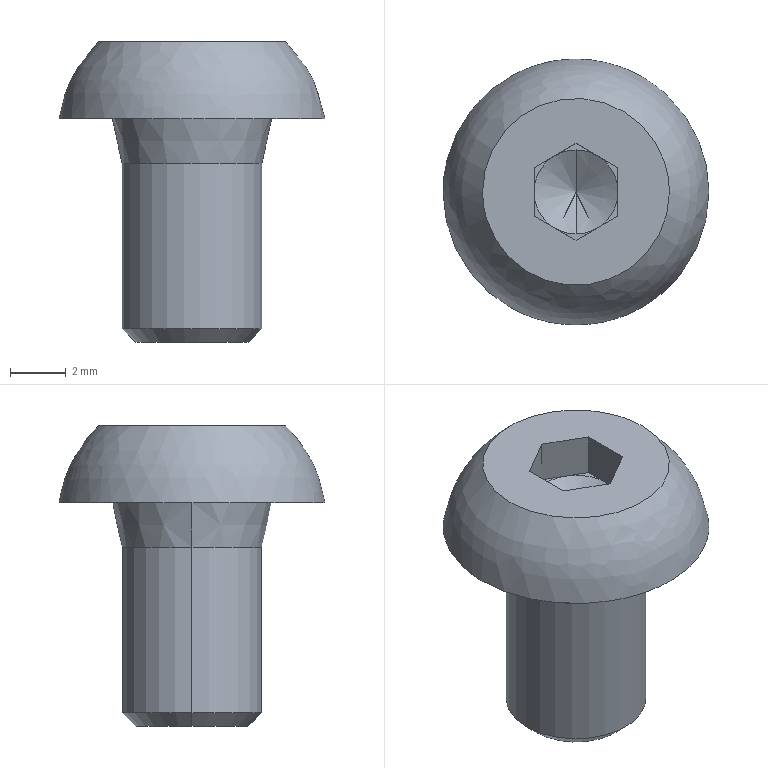Part | SolidWorks | features BaseBody 1 | 1 solid | 24 faces | box 9.5 x 9.5 x 10.75 mm | volume 302.249 mm3 | plane 15 | cone 6 | cylinder 2 | spline 1 | commonest cylinder face diameters 5 x2
STEP:
#1=CARTESIAN_POINT('',(2.5,0.,-5.91));
#2=VERTEX_POINT('',#1);
#3=CARTESIAN_POINT('',(-2.5,0.,-5.91));
#4=VERTEX_POINT('',#3);
#5=CARTESIAN_POINT('',(0.,0.,-5.91));
#6=DIRECTION('',(0.,0.,1.));
#7=DIRECTION('',(1.,0.,0.));
#8=AXIS2_PLACEMENT_3D('',#5,#6,#7);
#9=CIRCLE('',#8,2.5);
#10=EDGE_CURVE('',#2,#4,#9,.T.);
#11=ORIENTED_EDGE('',*,*,#10,.T.);
#12=CARTESIAN_POINT('',(-2.5,0.,0.));
#13=VERTEX_POINT('',#12);
#14=CARTESIAN_POINT('',(-2.5,0.,-6.4));
#15=DIRECTION('',(0.,0.,1.));
#16=VECTOR('',#15,1000.);
#17=LINE('',#14,#16);
#18=EDGE_CURVE('',#4,#13,#17,.T.);
#19=ORIENTED_EDGE('',*,*,#18,.T.);
#20=CARTESIAN_POINT('',(2.5,0.,0.));
#21=VERTEX_POINT('',#20);
#22=CARTESIAN_POINT('',(0.,0.,0.));
#23=DIRECTION('',(0.,0.,-1.));
#24=DIRECTION('',(1.,0.,0.));
#25=AXIS2_PLACEMENT_3D('',#22,#23,#24);
#26=CIRCLE('',#25,2.5);
#27=EDGE_CURVE('',#13,#21,#26,.T.);
#28=ORIENTED_EDGE('',*,*,#27,.T.);
#29=CARTESIAN_POINT('',(2.5,0.,-6.4));
#30=DIRECTION('',(0.,0.,1.));
#31=VECTOR('',#30,1000.);
#32=LINE('',#29,#31);
#33=EDGE_CURVE('',#2,#21,#32,.T.);
#34=ORIENTED_EDGE('',*,*,#33,.F.);
#35=EDGE_LOOP('',(#11,#19,#28,#34));
#36=FACE_OUTER_BOUND('',#35,.T.);
#37=CARTESIAN_POINT('',(0.,0.,-6.4));
#38=DIRECTION('',(0.,0.,1.));
#39=DIRECTION('',(1.,0.,0.));
#40=AXIS2_PLACEMENT_3D('',#37,#38,#39);
#41=CYLINDRICAL_SURFACE('',#40,2.5);
#42=ADVANCED_FACE('',(#36),#41,.T.);
#43=ORIENTED_EDGE('',*,*,#27,.F.);
#44=CARTESIAN_POINT('',(-2.85,0.,1.6));
#45=VERTEX_POINT('',#44);
#46=CARTESIAN_POINT('',(-2.85,0.,1.6));
#47=DIRECTION('',(-0.2137,0.,0.9769));
#48=VECTOR('',#47,1000.);
#49=LINE('',#46,#48);
#50=EDGE_CURVE('',#13,#45,#49,.T.);
#51=ORIENTED_EDGE('',*,*,#50,.T.);
#52=CARTESIAN_POINT('',(2.85,0.,1.6));
#53=VERTEX_POINT('',#52);
#54=CARTESIAN_POINT('',(0.,0.,1.6));
#55=DIRECTION('',(0.,0.,-1.));
#56=DIRECTION('',(1.,0.,0.));
#57=AXIS2_PLACEMENT_3D('',#54,#55,#56);
#58=CIRCLE('',#57,2.85);
#59=EDGE_CURVE('',#45,#53,#58,.T.);
#60=ORIENTED_EDGE('',*,*,#59,.T.);
#61=CARTESIAN_POINT('',(2.85,0.,1.6));
#62=DIRECTION('',(0.2137,0.,0.9769));
#63=VECTOR('',#62,1000.);
#64=LINE('',#61,#63);
#65=EDGE_CURVE('',#21,#53,#64,.T.);
#66=ORIENTED_EDGE('',*,*,#65,.F.);
#67=EDGE_LOOP('',(#43,#51,#60,#66));
#68=FACE_OUTER_BOUND('',#67,.T.);
#69=CARTESIAN_POINT('',(0.,0.,1.6));
#70=DIRECTION('',(0.,0.,1.));
#71=DIRECTION('',(1.,0.,0.));
#72=AXIS2_PLACEMENT_3D('',#69,#70,#71);
#73=CONICAL_SURFACE('',#72,2.85,0.2154);
#74=ADVANCED_FACE('',(#68),#73,.T.);
#75=CARTESIAN_POINT('',(2.009,0.,-6.4));
#76=VERTEX_POINT('',#75);
#77=CARTESIAN_POINT('',(-2.009,0.,-6.4));
#78=VERTEX_POINT('',#77);
#79=CARTESIAN_POINT('',(0.,0.,-6.4));
#80=DIRECTION('',(0.,0.,1.));
#81=DIRECTION('',(1.,0.,0.));
#82=AXIS2_PLACEMENT_3D('',#79,#80,#81);
#83=CIRCLE('',#82,2.009);
#84=EDGE_CURVE('',#76,#78,#83,.T.);
#85=ORIENTED_EDGE('',*,*,#84,.T.);
#86=CARTESIAN_POINT('',(-2.5,0.,-5.91));
#87=DIRECTION('',(-0.7071,0.,0.7071));
#88=VECTOR('',#87,1000.);
#89=LINE('',#86,#88);
#90=EDGE_CURVE('',#78,#4,#89,.T.);
#91=ORIENTED_EDGE('',*,*,#90,.T.);
#92=ORIENTED_EDGE('',*,*,#10,.F.);
#93=CARTESIAN_POINT('',(2.5,0.,-5.91));
#94=DIRECTION('',(0.7071,0.,0.7071));
#95=VECTOR('',#94,1000.);
#96=LINE('',#93,#95);
#97=EDGE_CURVE('',#76,#2,#96,.T.);
#98=ORIENTED_EDGE('',*,*,#97,.F.);
#99=EDGE_LOOP('',(#85,#91,#92,#98));
#100=FACE_OUTER_BOUND('',#99,.T.);
#101=CARTESIAN_POINT('',(0.,0.,-5.91));
#102=DIRECTION('',(0.,0.,1.));
#103=DIRECTION('',(1.,0.,0.));
#104=AXIS2_PLACEMENT_3D('',#101,#102,#103);
#105=CONICAL_SURFACE('',#104,2.5,0.7854);
#106=ADVANCED_FACE('',(#100),#105,.T.);
#107=CARTESIAN_POINT('',(0.,0.,1.924));
#108=VERTEX_POINT('',#107);
#109=CARTESIAN_POINT('',(0.,-1.5,2.79));
#110=VERTEX_POINT('',#109);
#111=CARTESIAN_POINT('',(0.,-1.5,2.79));
#112=DIRECTION('',(0.,-0.866,0.5));
#113=VECTOR('',#112,1000.);
#114=LINE('',#111,#113);
#115=EDGE_CURVE('',#108,#110,#114,.T.);
#116=ORIENTED_EDGE('',*,*,#115,.F.);
#117=CARTESIAN_POINT('',(0.,1.5,2.79));
#118=VERTEX_POINT('',#117);
#119=CARTESIAN_POINT('',(0.,1.5,2.79));
#120=DIRECTION('',(0.,0.866,0.5));
#121=VECTOR('',#120,1000.);
#122=LINE('',#119,#121);
#123=EDGE_CURVE('',#108,#118,#122,.T.);
#124=ORIENTED_EDGE('',*,*,#123,.T.);
#125=CARTESIAN_POINT('',(-0.75,1.299,2.79));
#126=VERTEX_POINT('',#125);
#127=CARTESIAN_POINT('',(0.,0.,2.79));
#128=DIRECTION('',(0.,0.,-1.));
#129=DIRECTION('',(0.,-1.,0.));
#130=AXIS2_PLACEMENT_3D('',#127,#128,#129);
#131=CIRCLE('',#130,1.5);
#132=EDGE_CURVE('',#126,#118,#131,.T.);
#133=ORIENTED_EDGE('',*,*,#132,.F.);
#134=CARTESIAN_POINT('',(-1.5,0.,2.79));
#135=VERTEX_POINT('',#134);
#136=CARTESIAN_POINT('',(0.,0.,2.79));
#137=DIRECTION('',(0.,0.,-1.));
#138=DIRECTION('',(0.,-1.,0.));
#139=AXIS2_PLACEMENT_3D('',#136,#137,#138);
#140=CIRCLE('',#139,1.5);
#141=EDGE_CURVE('',#135,#126,#140,.T.);
#142=ORIENTED_EDGE('',*,*,#141,.F.);
#143=CARTESIAN_POINT('',(-0.75,-1.299,2.79));
#144=VERTEX_POINT('',#143);
#145=CARTESIAN_POINT('',(0.,0.,2.79));
#146=DIRECTION('',(0.,0.,-1.));
#147=DIRECTION('',(0.,-1.,0.));
#148=AXIS2_PLACEMENT_3D('',#145,#146,#147);
#149=CIRCLE('',#148,1.5);
#150=EDGE_CURVE('',#144,#135,#149,.T.);
#151=ORIENTED_EDGE('',*,*,#150,.F.);
#152=CARTESIAN_POINT('',(0.,0.,2.79));
#153=DIRECTION('',(0.,0.,-1.));
#154=DIRECTION('',(0.,-1.,0.));
#155=AXIS2_PLACEMENT_3D('',#152,#153,#154);
#156=CIRCLE('',#155,1.5);
#157=EDGE_CURVE('',#110,#144,#156,.T.);
#158=ORIENTED_EDGE('',*,*,#157,.F.);
#159=EDGE_LOOP('',(#116,#124,#133,#142,#151,#158));
#160=FACE_OUTER_BOUND('',#159,.T.);
#161=CARTESIAN_POINT('',(0.,0.,2.79));
#162=DIRECTION('',(0.,0.,1.));
#163=DIRECTION('',(0.,-1.,0.));
#164=AXIS2_PLACEMENT_3D('',#161,#162,#163);
#165=CONICAL_SURFACE('',#164,1.5,1.047);
#166=ADVANCED_FACE('',(#160),#165,.F.);
#167=ORIENTED_EDGE('',*,*,#18,.F.);
#168=CARTESIAN_POINT('',(0.,0.,-5.91));
#169=DIRECTION('',(0.,0.,1.));
#170=DIRECTION('',(1.,0.,0.));
#171=AXIS2_PLACEMENT_3D('',#168,#169,#170);
#172=CIRCLE('',#171,2.5);
#173=EDGE_CURVE('',#4,#2,#172,.T.);
#174=ORIENTED_EDGE('',*,*,#173,.T.);
#175=ORIENTED_EDGE('',*,*,#33,.T.);
#176=CARTESIAN_POINT('',(0.,0.,0.));
#177=DIRECTION('',(0.,0.,-1.));
#178=DIRECTION('',(1.,0.,0.));
#179=AXIS2_PLACEMENT_3D('',#176,#177,#178);
#180=CIRCLE('',#179,2.5);
#181=EDGE_CURVE('',#21,#13,#180,.T.);
#182=ORIENTED_EDGE('',*,*,#181,.T.);
#183=EDGE_LOOP('',(#167,#174,#175,#182));
#184=FACE_OUTER_BOUND('',#183,.T.);
#185=CARTESIAN_POINT('',(0.,0.,-6.4));
#186=DIRECTION('',(0.,0.,1.));
#187=DIRECTION('',(1.,0.,0.));
#188=AXIS2_PLACEMENT_3D('',#185,#186,#187);
#189=CYLINDRICAL_SURFACE('',#188,2.5);
#190=ADVANCED_FACE('',(#184),#189,.T.);
#191=ORIENTED_EDGE('',*,*,#50,.F.);
#192=ORIENTED_EDGE('',*,*,#181,.F.);
#193=ORIENTED_EDGE('',*,*,#65,.T.);
#194=CARTESIAN_POINT('',(0.,0.,1.6));
#195=DIRECTION('',(0.,0.,-1.));
#196=DIRECTION('',(1.,0.,0.));
#197=AXIS2_PLACEMENT_3D('',#194,#195,#196);
#198=CIRCLE('',#197,2.85);
#199=EDGE_CURVE('',#53,#45,#198,.T.);
#200=ORIENTED_EDGE('',*,*,#199,.T.);
#201=EDGE_LOOP('',(#191,#192,#193,#200));
#202=FACE_OUTER_BOUND('',#201,.T.);
#203=CARTESIAN_POINT('',(0.,0.,1.6));
#204=DIRECTION('',(0.,0.,1.));
#205=DIRECTION('',(1.,0.,0.));
#206=AXIS2_PLACEMENT_3D('',#203,#204,#205);
#207=CONICAL_SURFACE('',#206,2.85,0.2154);
#208=ADVANCED_FACE('',(#202),#207,.T.);
#209=ORIENTED_EDGE('',*,*,#90,.F.);
#210=CARTESIAN_POINT('',(0.,0.,-6.4));
#211=DIRECTION('',(0.,0.,1.));
#212=DIRECTION('',(1.,0.,0.));
#213=AXIS2_PLACEMENT_3D('',#210,#211,#212);
#214=CIRCLE('',#213,2.009);
#215=EDGE_CURVE('',#78,#76,#214,.T.);
#216=ORIENTED_EDGE('',*,*,#215,.T.);
#217=ORIENTED_EDGE('',*,*,#97,.T.);
#218=ORIENTED_EDGE('',*,*,#173,.F.);
#219=EDGE_LOOP('',(#209,#216,#217,#218));
#220=FACE_OUTER_BOUND('',#219,.T.);
#221=CARTESIAN_POINT('',(0.,0.,-5.91));
#222=DIRECTION('',(0.,0.,1.));
#223=DIRECTION('',(1.,0.,0.));
#224=AXIS2_PLACEMENT_3D('',#221,#222,#223);
#225=CONICAL_SURFACE('',#224,2.5,0.7854);
#226=ADVANCED_FACE('',(#220),#225,.T.);
#227=CARTESIAN_POINT('',(-4.75,0.,1.6));
#228=VERTEX_POINT('',#227);
#229=CARTESIAN_POINT('',(4.75,-0.001679,1.6));
#230=VERTEX_POINT('',#229);
#231=CARTESIAN_POINT('',(-4.75,0.,1.6));
#232=CARTESIAN_POINT('',(-4.75,-0.3138,1.6));
#233=CARTESIAN_POINT('',(-4.719,-0.6224,1.6));
#234=CARTESIAN_POINT('',(-4.599,-1.229,1.6));
#235=CARTESIAN_POINT('',(-4.507,-1.531,1.6));
#236=CARTESIAN_POINT('',(-4.269,-2.106,1.6));
#237=CARTESIAN_POINT('',(-4.123,-2.379,1.6));
#238=CARTESIAN_POINT('',(-3.778,-2.895,1.6));
#239=CARTESIAN_POINT('',(-3.578,-3.14,1.6));
#240=CARTESIAN_POINT('',(-3.139,-3.578,1.6));
#241=CARTESIAN_POINT('',(-2.9,-3.775,1.6));
#242=CARTESIAN_POINT('',(-2.381,-4.122,1.6));
#243=CARTESIAN_POINT('',(-2.104,-4.27,1.6));
#244=CARTESIAN_POINT('',(-1.533,-4.506,1.6));
#245=CARTESIAN_POINT('',(-1.234,-4.598,1.6));
#246=CARTESIAN_POINT('',(-0.6205,-4.72,1.6));
#247=CARTESIAN_POINT('',(-0.3123,-4.75,1.6));
#248=CARTESIAN_POINT('',(0.3073,-4.75,1.6));
#249=CARTESIAN_POINT('',(0.6219,-4.719,1.6));
#250=CARTESIAN_POINT('',(1.231,-4.598,1.6));
#251=CARTESIAN_POINT('',(1.527,-4.509,1.6));
#252=CARTESIAN_POINT('',(2.102,-4.271,1.6));
#253=CARTESIAN_POINT('',(2.38,-4.122,1.6));
#254=CARTESIAN_POINT('',(2.895,-3.778,1.6));
#255=CARTESIAN_POINT('',(3.135,-3.582,1.6));
#256=CARTESIAN_POINT('',(3.579,-3.139,1.6));
#257=CARTESIAN_POINT('',(3.776,-2.899,1.6));
#258=CARTESIAN_POINT('',(4.12,-2.384,1.6));
#259=CARTESIAN_POINT('',(4.269,-2.107,1.6));
#260=CARTESIAN_POINT('',(4.507,-1.531,1.6));
#261=CARTESIAN_POINT('',(4.597,-1.235,1.6));
#262=CARTESIAN_POINT('',(4.719,-0.6265,1.6));
#263=CARTESIAN_POINT('',(4.75,-0.3117,1.6));
#264=CARTESIAN_POINT('',(4.75,-0.001679,1.6));
#265=B_SPLINE_CURVE_WITH_KNOTS('',3,(#231,#232,#233,#234,#235,#236,#237,#238,#239,#240,#241,#242,#243,#244,#245,#246,#247,#248,#249,#250,#251,#252,#253,#254,#255,#256,#257,#258,#259,#260,#261,#262,#263,#264),.UNSPECIFIED.,.F.,.F.,(4,2,2,2,2,2,2,2,2,2,2,2,2,2,2,2,4),(0.,0.0009281,0.001856,0.002784,0.003712,0.00464,0.005568,0.006496,0.007424,0.008353,0.009281,0.01021,0.01114,0.01206,0.01299,0.01392,0.01485),.UNSPECIFIED.);
#266=EDGE_CURVE('',#228,#230,#265,.T.);
#267=ORIENTED_EDGE('',*,*,#266,.F.);
#268=CARTESIAN_POINT('',(4.75,-0.001679,1.6));
#269=CARTESIAN_POINT('',(4.75,0.3083,1.6));
#270=CARTESIAN_POINT('',(4.72,0.6164,1.6));
#271=CARTESIAN_POINT('',(4.599,1.229,1.6));
#272=CARTESIAN_POINT('',(4.508,1.529,1.6));
#273=CARTESIAN_POINT('',(4.271,2.101,1.6));
#274=CARTESIAN_POINT('',(4.125,2.376,1.6));
#275=CARTESIAN_POINT('',(3.777,2.897,1.6));
#276=CARTESIAN_POINT('',(3.581,3.136,1.6));
#277=CARTESIAN_POINT('',(3.143,3.575,1.6));
#278=CARTESIAN_POINT('',(2.899,3.775,1.6));
#279=CARTESIAN_POINT('',(2.383,4.121,1.6));
#280=CARTESIAN_POINT('',(2.11,4.267,1.6));
#281=CARTESIAN_POINT('',(1.536,4.506,1.6));
#282=CARTESIAN_POINT('',(1.234,4.597,1.6));
#283=CARTESIAN_POINT('',(0.6264,4.719,1.6));
#284=CARTESIAN_POINT('',(0.318,4.75,1.6));
#285=CARTESIAN_POINT('',(-0.3084,4.75,1.6));
#286=CARTESIAN_POINT('',(-0.6184,4.72,1.6));
#287=CARTESIAN_POINT('',(-1.225,4.6,1.6));
#288=CARTESIAN_POINT('',(-1.526,4.509,1.6));
#289=CARTESIAN_POINT('',(-2.103,4.271,1.6));
#290=CARTESIAN_POINT('',(-2.376,4.125,1.6));
#291=CARTESIAN_POINT('',(-2.892,3.781,1.6));
#292=CARTESIAN_POINT('',(-3.137,3.581,1.6));
#293=CARTESIAN_POINT('',(-3.576,3.142,1.6));
#294=CARTESIAN_POINT('',(-3.772,2.903,1.6));
#295=CARTESIAN_POINT('',(-4.119,2.385,1.6));
#296=CARTESIAN_POINT('',(-4.268,2.108,1.6));
#297=CARTESIAN_POINT('',(-4.505,1.537,1.6));
#298=CARTESIAN_POINT('',(-4.596,1.239,1.6));
#299=CARTESIAN_POINT('',(-4.719,0.6244,1.6));
#300=CARTESIAN_POINT('',(-4.75,0.3138,1.6));
#301=CARTESIAN_POINT('',(-4.75,0.,1.6));
#302=B_SPLINE_CURVE_WITH_KNOTS('',3,(#268,#269,#270,#271,#272,#273,#274,#275,#276,#277,#278,#279,#280,#281,#282,#283,#284,#285,#286,#287,#288,#289,#290,#291,#292,#293,#294,#295,#296,#297,#298,#299,#300,#301),.UNSPECIFIED.,.F.,.F.,(4,2,2,2,2,2,2,2,2,2,2,2,2,2,2,2,4),(0.01485,0.01578,0.01671,0.01763,0.01856,0.01949,0.02042,0.02135,0.02227,0.0232,0.02413,0.02506,0.02599,0.02691,0.02784,0.02877,0.0297),.UNSPECIFIED.);
#303=EDGE_CURVE('',#230,#228,#302,.T.);
#304=ORIENTED_EDGE('',*,*,#303,.F.);
#305=EDGE_LOOP('',(#267,#304));
#306=FACE_OUTER_BOUND('',#305,.T.);
#307=ORIENTED_EDGE('',*,*,#199,.F.);
#308=ORIENTED_EDGE('',*,*,#59,.F.);
#309=EDGE_LOOP('',(#307,#308));
#310=FACE_BOUND('',#309,.T.);
#311=CARTESIAN_POINT('',(0.,4.75,1.6));
#312=DIRECTION('',(0.,0.,1.));
#313=DIRECTION('',(1.,0.,0.));
#314=AXIS2_PLACEMENT_3D('',#311,#312,#313);
#315=PLANE('',#314);
#316=ADVANCED_FACE('',(#306,#310),#315,.F.);
#317=ORIENTED_EDGE('',*,*,#84,.F.);
#318=ORIENTED_EDGE('',*,*,#215,.F.);
#319=EDGE_LOOP('',(#317,#318));
#320=FACE_OUTER_BOUND('',#319,.T.);
#321=CARTESIAN_POINT('',(0.,2.01,-6.4));
#322=DIRECTION('',(0.,0.,1.));
#323=DIRECTION('',(1.,0.,0.));
#324=AXIS2_PLACEMENT_3D('',#321,#322,#323);
#325=PLANE('',#324);
#326=ADVANCED_FACE('',(#320),#325,.F.);
#327=ORIENTED_EDGE('',*,*,#266,.T.);
#328=ORIENTED_EDGE('',*,*,#303,.T.);
#329=EDGE_LOOP('',(#327,#328));
#330=FACE_OUTER_BOUND('',#329,.T.);
#331=CARTESIAN_POINT('',(-3.339,0.,4.35));
#332=VERTEX_POINT('',#331);
#333=CARTESIAN_POINT('',(3.339,0.00118,4.35));
#334=VERTEX_POINT('',#333);
#335=CARTESIAN_POINT('',(-3.339,0.,4.35));
#336=CARTESIAN_POINT('',(-3.339,0.2206,4.35));
#337=CARTESIAN_POINT('',(-3.318,0.4375,4.35));
#338=CARTESIAN_POINT('',(-3.233,0.8643,4.35));
#339=CARTESIAN_POINT('',(-3.169,1.076,4.35));
#340=CARTESIAN_POINT('',(-3.001,1.481,4.35));
#341=CARTESIAN_POINT('',(-2.898,1.673,4.35));
#342=CARTESIAN_POINT('',(-2.656,2.035,4.35));
#343=CARTESIAN_POINT('',(-2.515,2.207,4.35));
#344=CARTESIAN_POINT('',(-2.207,2.515,4.35));
#345=CARTESIAN_POINT('',(-2.039,2.654,4.35));
#346=CARTESIAN_POINT('',(-1.674,2.898,4.35));
#347=CARTESIAN_POINT('',(-1.479,3.001,4.35));
#348=CARTESIAN_POINT('',(-1.078,3.168,4.35));
#349=CARTESIAN_POINT('',(-0.8672,3.232,4.35));
#350=CARTESIAN_POINT('',(-0.4362,3.318,4.35));
#351=CARTESIAN_POINT('',(-0.2195,3.339,4.35));
#352=CARTESIAN_POINT('',(0.216,3.339,4.35));
#353=CARTESIAN_POINT('',(0.4372,3.318,4.35));
#354=CARTESIAN_POINT('',(0.8654,3.232,4.35));
#355=CARTESIAN_POINT('',(1.074,3.169,4.35));
#356=CARTESIAN_POINT('',(1.478,3.002,4.35));
#357=CARTESIAN_POINT('',(1.673,2.898,4.35));
#358=CARTESIAN_POINT('',(2.035,2.656,4.35));
#359=CARTESIAN_POINT('',(2.204,2.518,4.35));
#360=CARTESIAN_POINT('',(2.516,2.207,4.35));
#361=CARTESIAN_POINT('',(2.654,2.038,4.35));
#362=CARTESIAN_POINT('',(2.896,1.676,4.35));
#363=CARTESIAN_POINT('',(3.001,1.481,4.35));
#364=CARTESIAN_POINT('',(3.169,1.076,4.35));
#365=CARTESIAN_POINT('',(3.232,0.8682,4.35));
#366=CARTESIAN_POINT('',(3.317,0.4404,4.35));
#367=CARTESIAN_POINT('',(3.339,0.2191,4.35));
#368=CARTESIAN_POINT('',(3.339,0.00118,4.35));
#369=B_SPLINE_CURVE_WITH_KNOTS('',3,(#335,#336,#337,#338,#339,#340,#341,#342,#343,#344,#345,#346,#347,#348,#349,#350,#351,#352,#353,#354,#355,#356,#357,#358,#359,#360,#361,#362,#363,#364,#365,#366,#367,#368),.UNSPECIFIED.,.F.,.F.,(4,2,2,2,2,2,2,2,2,2,2,2,2,2,2,2,4),(0.,0.0006524,0.001305,0.001957,0.00261,0.003262,0.003914,0.004567,0.005219,0.005872,0.006524,0.007177,0.007829,0.008481,0.009134,0.009786,0.01044),.UNSPECIFIED.);
#370=EDGE_CURVE('',#332,#334,#369,.T.);
#371=ORIENTED_EDGE('',*,*,#370,.T.);
#372=CARTESIAN_POINT('',(3.339,0.00118,4.35));
#373=CARTESIAN_POINT('',(3.339,-0.2167,4.35));
#374=CARTESIAN_POINT('',(3.318,-0.4333,4.35));
#375=CARTESIAN_POINT('',(3.233,-0.8637,4.35));
#376=CARTESIAN_POINT('',(3.169,-1.075,4.35));
#377=CARTESIAN_POINT('',(3.003,-1.477,4.35));
#378=CARTESIAN_POINT('',(2.9,-1.671,4.35));
#379=CARTESIAN_POINT('',(2.655,-2.036,4.35));
#380=CARTESIAN_POINT('',(2.517,-2.205,4.35));
#381=CARTESIAN_POINT('',(2.21,-2.513,4.35));
#382=CARTESIAN_POINT('',(2.038,-2.654,4.35));
#383=CARTESIAN_POINT('',(1.675,-2.897,4.35));
#384=CARTESIAN_POINT('',(1.483,-3.,4.35));
#385=CARTESIAN_POINT('',(1.08,-3.167,4.35));
#386=CARTESIAN_POINT('',(0.8672,-3.232,4.35));
#387=CARTESIAN_POINT('',(0.4403,-3.317,4.35));
#388=CARTESIAN_POINT('',(0.2236,-3.339,4.35));
#389=CARTESIAN_POINT('',(-0.2168,-3.339,4.35));
#390=CARTESIAN_POINT('',(-0.4347,-3.318,4.35));
#391=CARTESIAN_POINT('',(-0.8614,-3.233,4.35));
#392=CARTESIAN_POINT('',(-1.073,-3.17,4.35));
#393=CARTESIAN_POINT('',(-1.478,-3.002,4.35));
#394=CARTESIAN_POINT('',(-1.67,-2.9,4.35));
#395=CARTESIAN_POINT('',(-2.033,-2.658,4.35));
#396=CARTESIAN_POINT('',(-2.205,-2.517,4.35));
#397=CARTESIAN_POINT('',(-2.514,-2.209,4.35));
#398=CARTESIAN_POINT('',(-2.652,-2.041,4.35));
#399=CARTESIAN_POINT('',(-2.896,-1.677,4.35));
#400=CARTESIAN_POINT('',(-3.,-1.482,4.35));
#401=CARTESIAN_POINT('',(-3.25,-0.8795,4.35));
#402=CARTESIAN_POINT('',(-3.339,-0.4412,4.35));
#403=CARTESIAN_POINT('',(-3.339,0.,4.35));
#404=B_SPLINE_CURVE_WITH_KNOTS('',3,(#372,#373,#374,#375,#376,#377,#378,#379,#380,#381,#382,#383,#384,#385,#386,#387,#388,#389,#390,#391,#392,#393,#394,#395,#396,#397,#398,#399,#400,#401,#402,#403),.UNSPECIFIED.,.F.,.F.,(4,2,2,2,2,2,2,2,2,2,2,2,2,2,2,4),(0.01044,0.01109,0.01174,0.0124,0.01305,0.0137,0.01435,0.01501,0.01566,0.01631,0.01696,0.01762,0.01827,0.01892,0.01957,0.02088),.UNSPECIFIED.);
#405=EDGE_CURVE('',#334,#332,#404,.T.);
#406=ORIENTED_EDGE('',*,*,#405,.T.);
#407=EDGE_LOOP('',(#371,#406));
#408=FACE_BOUND('',#407,.T.);
#409=CARTESIAN_POINT('',(-0.5758,4.766,0.9748));
#410=CARTESIAN_POINT('',(-0.4577,4.766,1.884));
#411=CARTESIAN_POINT('',(0.4586,4.766,1.883));
#412=CARTESIAN_POINT('',(0.5759,4.766,0.9743));
#413=CARTESIAN_POINT('',(-8.271,3.821,1.975));
#414=CARTESIAN_POINT('',(-6.575,3.821,15.028));
#415=CARTESIAN_POINT('',(6.588,3.821,15.022));
#416=CARTESIAN_POINT('',(8.272,3.821,1.967));
#417=CARTESIAN_POINT('',(-8.189,-3.997,1.964));
#418=CARTESIAN_POINT('',(-6.51,-3.997,14.888));
#419=CARTESIAN_POINT('',(6.523,-3.997,14.882));
#420=CARTESIAN_POINT('',(8.19,-3.997,1.957));
#421=CARTESIAN_POINT('',(-0.4755,-4.777,0.9618));
#422=CARTESIAN_POINT('',(-0.378,-4.777,1.712));
#423=CARTESIAN_POINT('',(0.3787,-4.777,1.712));
#424=CARTESIAN_POINT('',(0.4755,-4.777,0.9613));
#425=(BOUNDED_SURFACE()B_SPLINE_SURFACE(3,3,((#409,#410,#411,#412),(#413,#414,#415,#416),(#417,#418,#419,#420),(#421,#422,#423,#424)),.UNSPECIFIED.,.F.,.F.,.F.)B_SPLINE_SURFACE_WITH_KNOTS((4,4),(4,4),(0.,1.),(0.,1.),.UNSPECIFIED.)GEOMETRIC_REPRESENTATION_ITEM()RATIONAL_B_SPLINE_SURFACE(((1.,0.4189,0.4189,1.),(0.4069,0.1705,0.1705,0.4069),(0.4069,0.1705,0.1705,0.4069),(1.,0.4189,0.4189,1.)))REPRESENTATION_ITEM('')SURFACE());
#426=ADVANCED_FACE('',(#330,#408),#425,.T.);
#427=CARTESIAN_POINT('',(-1.5,-0.866,4.35));
#428=VERTEX_POINT('',#427);
#429=CARTESIAN_POINT('',(0.,-1.732,4.35));
#430=VERTEX_POINT('',#429);
#431=CARTESIAN_POINT('',(-1.5,-0.866,4.35));
#432=DIRECTION('',(0.866,-0.5,0.));
#433=VECTOR('',#432,1000.);
#434=LINE('',#431,#433);
#435=EDGE_CURVE('',#428,#430,#434,.T.);
#436=ORIENTED_EDGE('',*,*,#435,.F.);
#437=CARTESIAN_POINT('',(-1.5,0.866,4.35));
#438=VERTEX_POINT('',#437);
#439=CARTESIAN_POINT('',(-1.5,0.,4.35));
#440=DIRECTION('',(0.,-1.,0.));
#441=VECTOR('',#440,1000.);
#442=LINE('',#439,#441);
#443=EDGE_CURVE('',#438,#428,#442,.T.);
#444=ORIENTED_EDGE('',*,*,#443,.F.);
#445=CARTESIAN_POINT('',(0.,1.732,4.35));
#446=VERTEX_POINT('',#445);
#447=CARTESIAN_POINT('',(0.,1.732,4.35));
#448=DIRECTION('',(-0.866,-0.5,0.));
#449=VECTOR('',#448,1000.);
#450=LINE('',#447,#449);
#451=EDGE_CURVE('',#446,#438,#450,.T.);
#452=ORIENTED_EDGE('',*,*,#451,.F.);
#453=CARTESIAN_POINT('',(1.5,0.866,4.35));
#454=VERTEX_POINT('',#453);
#455=CARTESIAN_POINT('',(1.5,0.866,4.35));
#456=DIRECTION('',(-0.866,0.5,0.));
#457=VECTOR('',#456,1000.);
#458=LINE('',#455,#457);
#459=EDGE_CURVE('',#454,#446,#458,.T.);
#460=ORIENTED_EDGE('',*,*,#459,.F.);
#461=CARTESIAN_POINT('',(1.5,-0.866,4.35));
#462=VERTEX_POINT('',#461);
#463=CARTESIAN_POINT('',(1.5,0.,4.35));
#464=DIRECTION('',(0.,1.,0.));
#465=VECTOR('',#464,1000.);
#466=LINE('',#463,#465);
#467=EDGE_CURVE('',#462,#454,#466,.T.);
#468=ORIENTED_EDGE('',*,*,#467,.F.);
#469=CARTESIAN_POINT('',(0.,-1.732,4.35));
#470=DIRECTION('',(0.866,0.5,0.));
#471=VECTOR('',#470,1000.);
#472=LINE('',#469,#471);
#473=EDGE_CURVE('',#430,#462,#472,.T.);
#474=ORIENTED_EDGE('',*,*,#473,.F.);
#475=EDGE_LOOP('',(#436,#444,#452,#460,#468,#474));
#476=FACE_BOUND('',#475,.T.);
#477=ORIENTED_EDGE('',*,*,#370,.F.);
#478=ORIENTED_EDGE('',*,*,#405,.F.);
#479=EDGE_LOOP('',(#477,#478));
#480=FACE_OUTER_BOUND('',#479,.T.);
#481=CARTESIAN_POINT('',(0.,0.,4.35));
#482=DIRECTION('',(0.,0.,-1.));
#483=DIRECTION('',(-1.,0.,0.));
#484=AXIS2_PLACEMENT_3D('',#481,#482,#483);
#485=PLANE('',#484);
#486=ADVANCED_FACE('',(#476,#480),#485,.F.);
#487=CARTESIAN_POINT('',(1.5,-0.866,2.79));
#488=VERTEX_POINT('',#487);
#489=CARTESIAN_POINT('',(1.5,-0.866,2.79));
#490=DIRECTION('',(0.,0.,1.));
#491=VECTOR('',#490,1000.);
#492=LINE('',#489,#491);
#493=EDGE_CURVE('',#488,#462,#492,.T.);
#494=ORIENTED_EDGE('',*,*,#493,.F.);
#495=CARTESIAN_POINT('',(0.75,-1.299,2.79));
#496=VERTEX_POINT('',#495);
#497=CARTESIAN_POINT('',(0.,-1.732,2.79));
#498=DIRECTION('',(0.866,0.5,0.));
#499=VECTOR('',#498,1000.);
#500=LINE('',#497,#499);
#501=EDGE_CURVE('',#496,#488,#500,.T.);
#502=ORIENTED_EDGE('',*,*,#501,.F.);
#503=CARTESIAN_POINT('',(0.,-1.732,2.79));
#504=VERTEX_POINT('',#503);
#505=CARTESIAN_POINT('',(0.,-1.732,2.79));
#506=DIRECTION('',(0.866,0.5,0.));
#507=VECTOR('',#506,1000.);
#508=LINE('',#505,#507);
#509=EDGE_CURVE('',#504,#496,#508,.T.);
#510=ORIENTED_EDGE('',*,*,#509,.F.);
#511=CARTESIAN_POINT('',(0.,-1.732,2.79));
#512=DIRECTION('',(0.,0.,-1.));
#513=VECTOR('',#512,1000.);
#514=LINE('',#511,#513);
#515=EDGE_CURVE('',#430,#504,#514,.T.);
#516=ORIENTED_EDGE('',*,*,#515,.F.);
#517=ORIENTED_EDGE('',*,*,#473,.T.);
#518=EDGE_LOOP('',(#494,#502,#510,#516,#517));
#519=FACE_OUTER_BOUND('',#518,.T.);
#520=CARTESIAN_POINT('',(0.,-1.732,2.79));
#521=DIRECTION('',(0.5,-0.866,0.));
#522=DIRECTION('',(0.866,0.5,0.));
#523=AXIS2_PLACEMENT_3D('',#520,#521,#522);
#524=PLANE('',#523);
#525=ADVANCED_FACE('',(#519),#524,.F.);
#526=ORIENTED_EDGE('',*,*,#515,.T.);
#527=CARTESIAN_POINT('',(-1.5,-0.866,2.79));
#528=DIRECTION('',(0.866,-0.5,0.));
#529=VECTOR('',#528,1000.);
#530=LINE('',#527,#529);
#531=EDGE_CURVE('',#144,#504,#530,.T.);
#532=ORIENTED_EDGE('',*,*,#531,.F.);
#533=CARTESIAN_POINT('',(-1.5,-0.866,2.79));
#534=VERTEX_POINT('',#533);
#535=CARTESIAN_POINT('',(-1.5,-0.866,2.79));
#536=DIRECTION('',(0.866,-0.5,0.));
#537=VECTOR('',#536,1000.);
#538=LINE('',#535,#537);
#539=EDGE_CURVE('',#534,#144,#538,.T.);
#540=ORIENTED_EDGE('',*,*,#539,.F.);
#541=CARTESIAN_POINT('',(-1.5,-0.866,2.79));
#542=DIRECTION('',(0.,0.,-1.));
#543=VECTOR('',#542,1000.);
#544=LINE('',#541,#543);
#545=EDGE_CURVE('',#428,#534,#544,.T.);
#546=ORIENTED_EDGE('',*,*,#545,.F.);
#547=ORIENTED_EDGE('',*,*,#435,.T.);
#548=EDGE_LOOP('',(#526,#532,#540,#546,#547));
#549=FACE_OUTER_BOUND('',#548,.T.);
#550=CARTESIAN_POINT('',(-1.5,-0.866,2.79));
#551=DIRECTION('',(-0.5,-0.866,0.));
#552=DIRECTION('',(0.866,-0.5,0.));
#553=AXIS2_PLACEMENT_3D('',#550,#551,#552);
#554=PLANE('',#553);
#555=ADVANCED_FACE('',(#549),#554,.F.);
#556=ORIENTED_EDGE('',*,*,#545,.T.);
#557=CARTESIAN_POINT('',(-1.5,0.866,2.79));
#558=DIRECTION('',(0.,-1.,0.));
#559=VECTOR('',#558,1000.);
#560=LINE('',#557,#559);
#561=EDGE_CURVE('',#135,#534,#560,.T.);
#562=ORIENTED_EDGE('',*,*,#561,.F.);
#563=CARTESIAN_POINT('',(-1.5,0.866,2.79));
#564=VERTEX_POINT('',#563);
#565=CARTESIAN_POINT('',(-1.5,0.866,2.79));
#566=DIRECTION('',(0.,-1.,0.));
#567=VECTOR('',#566,1000.);
#568=LINE('',#565,#567);
#569=EDGE_CURVE('',#564,#135,#568,.T.);
#570=ORIENTED_EDGE('',*,*,#569,.F.);
#571=CARTESIAN_POINT('',(-1.5,0.866,2.79));
#572=DIRECTION('',(0.,0.,-1.));
#573=VECTOR('',#572,1000.);
#574=LINE('',#571,#573);
#575=EDGE_CURVE('',#438,#564,#574,.T.);
#576=ORIENTED_EDGE('',*,*,#575,.F.);
#577=ORIENTED_EDGE('',*,*,#443,.T.);
#578=EDGE_LOOP('',(#556,#562,#570,#576,#577));
#579=FACE_OUTER_BOUND('',#578,.T.);
#580=CARTESIAN_POINT('',(-1.5,0.866,2.79));
#581=DIRECTION('',(-1.,0.,0.));
#582=DIRECTION('',(0.,0.,1.));
#583=AXIS2_PLACEMENT_3D('',#580,#581,#582);
#584=PLANE('',#583);
#585=ADVANCED_FACE('',(#579),#584,.F.);
#586=ORIENTED_EDGE('',*,*,#575,.T.);
#587=CARTESIAN_POINT('',(0.,1.732,2.79));
#588=DIRECTION('',(-0.866,-0.5,0.));
#589=VECTOR('',#588,1000.);
#590=LINE('',#587,#589);
#591=EDGE_CURVE('',#126,#564,#590,.T.);
#592=ORIENTED_EDGE('',*,*,#591,.F.);
#593=CARTESIAN_POINT('',(0.,1.732,2.79));
#594=VERTEX_POINT('',#593);
#595=CARTESIAN_POINT('',(0.,1.732,2.79));
#596=DIRECTION('',(-0.866,-0.5,0.));
#597=VECTOR('',#596,1000.);
#598=LINE('',#595,#597);
#599=EDGE_CURVE('',#594,#126,#598,.T.);
#600=ORIENTED_EDGE('',*,*,#599,.F.);
#601=CARTESIAN_POINT('',(0.,1.732,2.79));
#602=DIRECTION('',(0.,0.,-1.));
#603=VECTOR('',#602,1000.);
#604=LINE('',#601,#603);
#605=EDGE_CURVE('',#446,#594,#604,.T.);
#606=ORIENTED_EDGE('',*,*,#605,.F.);
#607=ORIENTED_EDGE('',*,*,#451,.T.);
#608=EDGE_LOOP('',(#586,#592,#600,#606,#607));
#609=FACE_OUTER_BOUND('',#608,.T.);
#610=CARTESIAN_POINT('',(0.,1.732,2.79));
#611=DIRECTION('',(-0.5,0.866,0.));
#612=DIRECTION('',(-0.866,-0.5,0.));
#613=AXIS2_PLACEMENT_3D('',#610,#611,#612);
#614=PLANE('',#613);
#615=ADVANCED_FACE('',(#609),#614,.F.);
#616=ORIENTED_EDGE('',*,*,#605,.T.);
#617=CARTESIAN_POINT('',(0.75,1.299,2.79));
#618=VERTEX_POINT('',#617);
#619=CARTESIAN_POINT('',(1.5,0.866,2.79));
#620=DIRECTION('',(-0.866,0.5,0.));
#621=VECTOR('',#620,1000.);
#622=LINE('',#619,#621);
#623=EDGE_CURVE('',#618,#594,#622,.T.);
#624=ORIENTED_EDGE('',*,*,#623,.F.);
#625=CARTESIAN_POINT('',(1.5,0.866,2.79));
#626=VERTEX_POINT('',#625);
#627=CARTESIAN_POINT('',(1.5,0.866,2.79));
#628=DIRECTION('',(-0.866,0.5,0.));
#629=VECTOR('',#628,1000.);
#630=LINE('',#627,#629);
#631=EDGE_CURVE('',#626,#618,#630,.T.);
#632=ORIENTED_EDGE('',*,*,#631,.F.);
#633=CARTESIAN_POINT('',(1.5,0.866,2.79));
#634=DIRECTION('',(0.,0.,-1.));
#635=VECTOR('',#634,1000.);
#636=LINE('',#633,#635);
#637=EDGE_CURVE('',#454,#626,#636,.T.);
#638=ORIENTED_EDGE('',*,*,#637,.F.);
#639=ORIENTED_EDGE('',*,*,#459,.T.);
#640=EDGE_LOOP('',(#616,#624,#632,#638,#639));
#641=FACE_OUTER_BOUND('',#640,.T.);
#642=CARTESIAN_POINT('',(1.5,0.866,2.79));
#643=DIRECTION('',(0.5,0.866,0.));
#644=DIRECTION('',(-0.866,0.5,0.));
#645=AXIS2_PLACEMENT_3D('',#642,#643,#644);
#646=PLANE('',#645);
#647=ADVANCED_FACE('',(#641),#646,.F.);
#648=ORIENTED_EDGE('',*,*,#637,.T.);
#649=CARTESIAN_POINT('',(1.5,0.,2.79));
#650=VERTEX_POINT('',#649);
#651=CARTESIAN_POINT('',(1.5,-0.866,2.79));
#652=DIRECTION('',(0.,1.,0.));
#653=VECTOR('',#652,1000.);
#654=LINE('',#651,#653);
#655=EDGE_CURVE('',#650,#626,#654,.T.);
#656=ORIENTED_EDGE('',*,*,#655,.F.);
#657=CARTESIAN_POINT('',(1.5,-0.866,2.79));
#658=DIRECTION('',(0.,1.,0.));
#659=VECTOR('',#658,1000.);
#660=LINE('',#657,#659);
#661=EDGE_CURVE('',#488,#650,#660,.T.);
#662=ORIENTED_EDGE('',*,*,#661,.F.);
#663=ORIENTED_EDGE('',*,*,#493,.T.);
#664=ORIENTED_EDGE('',*,*,#467,.T.);
#665=EDGE_LOOP('',(#648,#656,#662,#663,#664));
#666=FACE_OUTER_BOUND('',#665,.T.);
#667=CARTESIAN_POINT('',(1.5,-0.866,2.79));
#668=DIRECTION('',(1.,0.,0.));
#669=DIRECTION('',(0.,0.,-1.));
#670=AXIS2_PLACEMENT_3D('',#667,#668,#669);
#671=PLANE('',#670);
#672=ADVANCED_FACE('',(#666),#671,.F.);
#673=CARTESIAN_POINT('',(0.,0.,2.79));
#674=DIRECTION('',(0.,0.,-1.));
#675=DIRECTION('',(0.,-1.,0.));
#676=AXIS2_PLACEMENT_3D('',#673,#674,#675);
#677=CIRCLE('',#676,1.5);
#678=EDGE_CURVE('',#650,#496,#677,.T.);
#679=ORIENTED_EDGE('',*,*,#678,.T.);
#680=ORIENTED_EDGE('',*,*,#501,.T.);
#681=ORIENTED_EDGE('',*,*,#661,.T.);
#682=EDGE_LOOP('',(#679,#680,#681));
#683=FACE_OUTER_BOUND('',#682,.T.);
#684=CARTESIAN_POINT('',(0.,0.,2.79));
#685=DIRECTION('',(0.,0.,1.));
#686=DIRECTION('',(1.,0.,0.));
#687=AXIS2_PLACEMENT_3D('',#684,#685,#686);
#688=PLANE('',#687);
#689=ADVANCED_FACE('',(#683),#688,.T.);
#690=CARTESIAN_POINT('',(0.,0.,2.79));
#691=DIRECTION('',(0.,0.,-1.));
#692=DIRECTION('',(0.,-1.,0.));
#693=AXIS2_PLACEMENT_3D('',#690,#691,#692);
#694=CIRCLE('',#693,1.5);
#695=EDGE_CURVE('',#496,#110,#694,.T.);
#696=ORIENTED_EDGE('',*,*,#695,.T.);
#697=ORIENTED_EDGE('',*,*,#157,.T.);
#698=ORIENTED_EDGE('',*,*,#531,.T.);
#699=ORIENTED_EDGE('',*,*,#509,.T.);
#700=EDGE_LOOP('',(#696,#697,#698,#699));
#701=FACE_OUTER_BOUND('',#700,.T.);
#702=CARTESIAN_POINT('',(0.,0.,2.79));
#703=DIRECTION('',(0.,0.,1.));
#704=DIRECTION('',(1.,0.,0.));
#705=AXIS2_PLACEMENT_3D('',#702,#703,#704);
#706=PLANE('',#705);
#707=ADVANCED_FACE('',(#701),#706,.T.);
#708=ORIENTED_EDGE('',*,*,#150,.T.);
#709=ORIENTED_EDGE('',*,*,#561,.T.);
#710=ORIENTED_EDGE('',*,*,#539,.T.);
#711=EDGE_LOOP('',(#708,#709,#710));
#712=FACE_OUTER_BOUND('',#711,.T.);
#713=CARTESIAN_POINT('',(0.,0.,2.79));
#714=DIRECTION('',(0.,0.,1.));
#715=DIRECTION('',(1.,0.,0.));
#716=AXIS2_PLACEMENT_3D('',#713,#714,#715);
#717=PLANE('',#716);
#718=ADVANCED_FACE('',(#712),#717,.T.);
#719=ORIENTED_EDGE('',*,*,#141,.T.);
#720=ORIENTED_EDGE('',*,*,#591,.T.);
#721=ORIENTED_EDGE('',*,*,#569,.T.);
#722=EDGE_LOOP('',(#719,#720,#721));
#723=FACE_OUTER_BOUND('',#722,.T.);
#724=CARTESIAN_POINT('',(0.,0.,2.79));
#725=DIRECTION('',(0.,0.,1.));
#726=DIRECTION('',(1.,0.,0.));
#727=AXIS2_PLACEMENT_3D('',#724,#725,#726);
#728=PLANE('',#727);
#729=ADVANCED_FACE('',(#723),#728,.T.);
#730=ORIENTED_EDGE('',*,*,#132,.T.);
#731=CARTESIAN_POINT('',(0.,0.,2.79));
#732=DIRECTION('',(0.,0.,-1.));
#733=DIRECTION('',(0.,-1.,0.));
#734=AXIS2_PLACEMENT_3D('',#731,#732,#733);
#735=CIRCLE('',#734,1.5);
#736=EDGE_CURVE('',#118,#618,#735,.T.);
#737=ORIENTED_EDGE('',*,*,#736,.T.);
#738=ORIENTED_EDGE('',*,*,#623,.T.);
#739=ORIENTED_EDGE('',*,*,#599,.T.);
#740=EDGE_LOOP('',(#730,#737,#738,#739));
#741=FACE_OUTER_BOUND('',#740,.T.);
#742=CARTESIAN_POINT('',(0.,0.,2.79));
#743=DIRECTION('',(0.,0.,1.));
#744=DIRECTION('',(1.,0.,0.));
#745=AXIS2_PLACEMENT_3D('',#742,#743,#744);
#746=PLANE('',#745);
#747=ADVANCED_FACE('',(#741),#746,.T.);
#748=CARTESIAN_POINT('',(0.,0.,2.79));
#749=DIRECTION('',(0.,0.,-1.));
#750=DIRECTION('',(0.,-1.,0.));
#751=AXIS2_PLACEMENT_3D('',#748,#749,#750);
#752=CIRCLE('',#751,1.5);
#753=EDGE_CURVE('',#618,#650,#752,.T.);
#754=ORIENTED_EDGE('',*,*,#753,.T.);
#755=ORIENTED_EDGE('',*,*,#655,.T.);
#756=ORIENTED_EDGE('',*,*,#631,.T.);
#757=EDGE_LOOP('',(#754,#755,#756));
#758=FACE_OUTER_BOUND('',#757,.T.);
#759=CARTESIAN_POINT('',(0.,0.,2.79));
#760=DIRECTION('',(0.,0.,1.));
#761=DIRECTION('',(1.,0.,0.));
#762=AXIS2_PLACEMENT_3D('',#759,#760,#761);
#763=PLANE('',#762);
#764=ADVANCED_FACE('',(#758),#763,.T.);
#765=ORIENTED_EDGE('',*,*,#123,.F.);
#766=ORIENTED_EDGE('',*,*,#115,.T.);
#767=ORIENTED_EDGE('',*,*,#695,.F.);
#768=ORIENTED_EDGE('',*,*,#678,.F.);
#769=ORIENTED_EDGE('',*,*,#753,.F.);
#770=ORIENTED_EDGE('',*,*,#736,.F.);
#771=EDGE_LOOP('',(#765,#766,#767,#768,#769,#770));
#772=FACE_OUTER_BOUND('',#771,.T.);
#773=CARTESIAN_POINT('',(0.,0.,2.79));
#774=DIRECTION('',(0.,0.,1.));
#775=DIRECTION('',(0.,-1.,0.));
#776=AXIS2_PLACEMENT_3D('',#773,#774,#775);
#777=CONICAL_SURFACE('',#776,1.5,1.047);
#778=ADVANCED_FACE('',(#772),#777,.F.);
#779=CLOSED_SHELL('',(#42,#74,#106,#166,#190,#208,#226,#316,#326,#426,#486,#525,#555,#585,#615,#647,#672,#689,#707,#718,#729,#747,#764,#778));
#780=MANIFOLD_SOLID_BREP('',#779);
#781=CARTESIAN_POINT('',(0.,0.,0.));
#782=DIRECTION('',(0.,0.,1.));
#783=DIRECTION('',(1.,0.,0.));
#784=AXIS2_PLACEMENT_3D('',#781,#782,#783);
#785=(LENGTH_UNIT()NAMED_UNIT(*)SI_UNIT(.MILLI.,.METRE.));
#786=UNCERTAINTY_MEASURE_WITH_UNIT(LENGTH_MEASURE(0.00001),#785,'','');
#787=(NAMED_UNIT(*)PLANE_ANGLE_UNIT()SI_UNIT($,.RADIAN.));
#788=(NAMED_UNIT(*)SI_UNIT($,.STERADIAN.)SOLID_ANGLE_UNIT());
#789=(GEOMETRIC_REPRESENTATION_CONTEXT(3)GLOBAL_UNCERTAINTY_ASSIGNED_CONTEXT((#786))GLOBAL_UNIT_ASSIGNED_CONTEXT((#785,#787,#788))REPRESENTATION_CONTEXT('',''));
#790=ADVANCED_BREP_SHAPE_REPRESENTATION('',(#780,#784),#789);